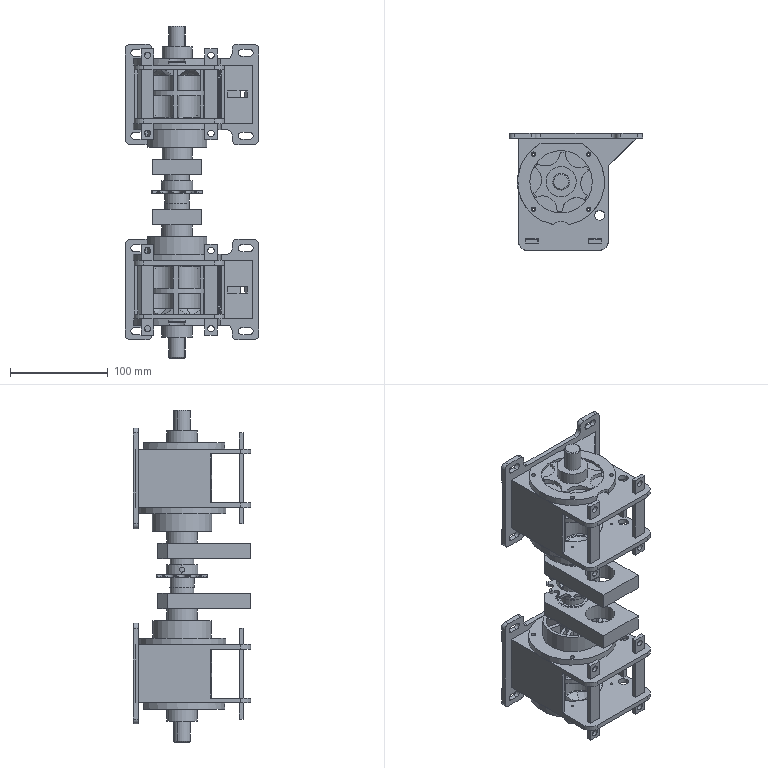Part | NX | features EXTRUDE 18, DATUM_CSYS 12, SKETCH 12, BREP 7, EXTRACT_DATUM_PLANE 6, LINKED_FACE 4, EXTRACT_BODY 3, UNITE 3, DATUM_PLANE 1, Delete Body 1, INTERSECT 1, Pattern Geometry 1, REPLACE_FACE 1 | 33 solids | 1138 faces | box 136.5 x 120 x 340 mm | volume 908883 mm3 | plane 593 | cylinder 401 | sphere 60 | cone 56 | torus 28 | commonest cylinder face diameters 30 x66 17 x36 2.5 x32 61 x26 10 x24 54 x24